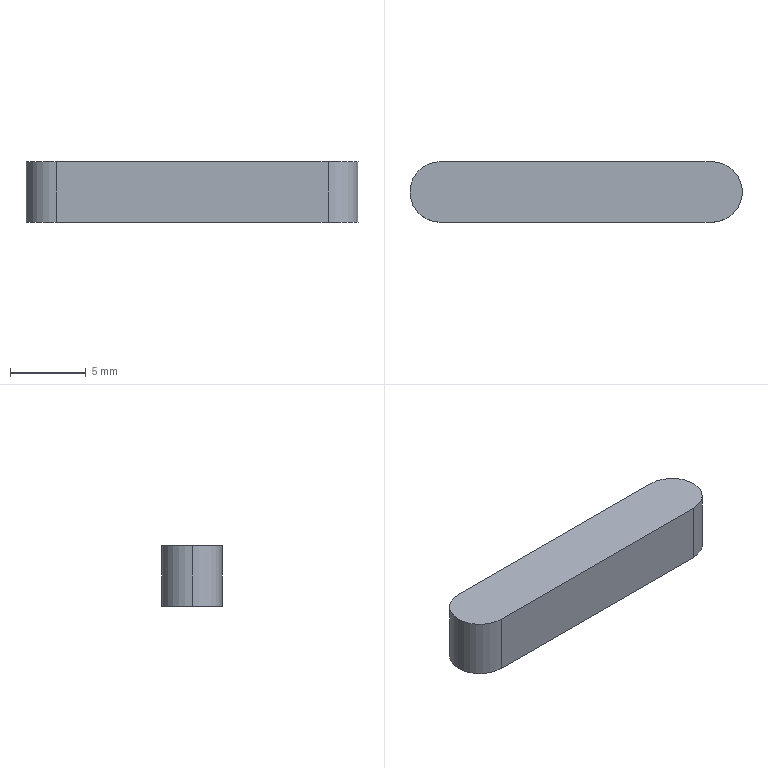Part | SolidWorks | features Extrusion 1 | 1 solid | 7 faces | box 22 x 4 x 4 mm | volume 338.265 mm3 | plane 4 | cylinder 3 | commonest cylinder face diameters 4 x3
STEP:
#1=CARTESIAN_POINT('',(-2.,0.,4.));
#2=VERTEX_POINT('',#1);
#3=CARTESIAN_POINT('',(0.,-2.,4.));
#4=VERTEX_POINT('',#3);
#5=CARTESIAN_POINT('',(0.,0.,4.));
#6=DIRECTION('',(0.,0.,1.));
#7=DIRECTION('',(1.,0.,0.));
#8=AXIS2_PLACEMENT_3D('',#5,#6,#7);
#9=CIRCLE('',#8,2.);
#10=EDGE_CURVE('',#2,#4,#9,.T.);
#11=ORIENTED_EDGE('',*,*,#10,.F.);
#12=CARTESIAN_POINT('',(-2.,0.,0.));
#13=VERTEX_POINT('',#12);
#14=CARTESIAN_POINT('',(-2.,0.,4.));
#15=DIRECTION('',(0.,0.,-1.));
#16=VECTOR('',#15,1000.);
#17=LINE('',#14,#16);
#18=EDGE_CURVE('',#2,#13,#17,.T.);
#19=ORIENTED_EDGE('',*,*,#18,.T.);
#20=CARTESIAN_POINT('',(0.,-2.,0.));
#21=VERTEX_POINT('',#20);
#22=CARTESIAN_POINT('',(0.,0.,0.));
#23=DIRECTION('',(0.,0.,1.));
#24=DIRECTION('',(1.,0.,0.));
#25=AXIS2_PLACEMENT_3D('',#22,#23,#24);
#26=CIRCLE('',#25,2.);
#27=EDGE_CURVE('',#13,#21,#26,.T.);
#28=ORIENTED_EDGE('',*,*,#27,.T.);
#29=CARTESIAN_POINT('',(0.,-2.,4.));
#30=DIRECTION('',(0.,0.,-1.));
#31=VECTOR('',#30,1000.);
#32=LINE('',#29,#31);
#33=EDGE_CURVE('',#4,#21,#32,.T.);
#34=ORIENTED_EDGE('',*,*,#33,.F.);
#35=EDGE_LOOP('',(#11,#19,#28,#34));
#36=FACE_OUTER_BOUND('',#35,.T.);
#37=CARTESIAN_POINT('',(0.,0.,4.));
#38=DIRECTION('',(0.,0.,-1.));
#39=DIRECTION('',(-1.,0.,0.));
#40=AXIS2_PLACEMENT_3D('',#37,#38,#39);
#41=CYLINDRICAL_SURFACE('',#40,2.);
#42=ADVANCED_FACE('',(#36),#41,.T.);
#43=ORIENTED_EDGE('',*,*,#18,.F.);
#44=CARTESIAN_POINT('',(0.,2.,4.));
#45=VERTEX_POINT('',#44);
#46=CARTESIAN_POINT('',(0.,0.,4.));
#47=DIRECTION('',(0.,0.,1.));
#48=DIRECTION('',(1.,0.,0.));
#49=AXIS2_PLACEMENT_3D('',#46,#47,#48);
#50=CIRCLE('',#49,2.);
#51=EDGE_CURVE('',#45,#2,#50,.T.);
#52=ORIENTED_EDGE('',*,*,#51,.F.);
#53=CARTESIAN_POINT('',(0.,2.,0.));
#54=VERTEX_POINT('',#53);
#55=CARTESIAN_POINT('',(0.,2.,4.));
#56=DIRECTION('',(0.,0.,-1.));
#57=VECTOR('',#56,1000.);
#58=LINE('',#55,#57);
#59=EDGE_CURVE('',#45,#54,#58,.T.);
#60=ORIENTED_EDGE('',*,*,#59,.T.);
#61=CARTESIAN_POINT('',(0.,0.,0.));
#62=DIRECTION('',(0.,0.,1.));
#63=DIRECTION('',(1.,0.,0.));
#64=AXIS2_PLACEMENT_3D('',#61,#62,#63);
#65=CIRCLE('',#64,2.);
#66=EDGE_CURVE('',#54,#13,#65,.T.);
#67=ORIENTED_EDGE('',*,*,#66,.T.);
#68=EDGE_LOOP('',(#43,#52,#60,#67));
#69=FACE_OUTER_BOUND('',#68,.T.);
#70=CARTESIAN_POINT('',(0.,0.,4.));
#71=DIRECTION('',(0.,0.,-1.));
#72=DIRECTION('',(-1.,0.,0.));
#73=AXIS2_PLACEMENT_3D('',#70,#71,#72);
#74=CYLINDRICAL_SURFACE('',#73,2.);
#75=ADVANCED_FACE('',(#69),#74,.T.);
#76=CARTESIAN_POINT('',(18.,-2.,0.));
#77=VERTEX_POINT('',#76);
#78=CARTESIAN_POINT('',(0.,-2.,0.));
#79=DIRECTION('',(1.,0.,0.));
#80=VECTOR('',#79,1000.);
#81=LINE('',#78,#80);
#82=EDGE_CURVE('',#21,#77,#81,.T.);
#83=ORIENTED_EDGE('',*,*,#82,.T.);
#84=CARTESIAN_POINT('',(18.,-2.,4.));
#85=VERTEX_POINT('',#84);
#86=CARTESIAN_POINT('',(18.,-2.,4.));
#87=DIRECTION('',(0.,0.,-1.));
#88=VECTOR('',#87,1000.);
#89=LINE('',#86,#88);
#90=EDGE_CURVE('',#85,#77,#89,.T.);
#91=ORIENTED_EDGE('',*,*,#90,.F.);
#92=CARTESIAN_POINT('',(0.,-2.,4.));
#93=DIRECTION('',(1.,0.,0.));
#94=VECTOR('',#93,1000.);
#95=LINE('',#92,#94);
#96=EDGE_CURVE('',#4,#85,#95,.T.);
#97=ORIENTED_EDGE('',*,*,#96,.F.);
#98=ORIENTED_EDGE('',*,*,#33,.T.);
#99=EDGE_LOOP('',(#83,#91,#97,#98));
#100=FACE_OUTER_BOUND('',#99,.T.);
#101=CARTESIAN_POINT('',(0.,-2.,4.));
#102=DIRECTION('',(0.,1.,0.));
#103=DIRECTION('',(0.,0.,1.));
#104=AXIS2_PLACEMENT_3D('',#101,#102,#103);
#105=PLANE('',#104);
#106=ADVANCED_FACE('',(#100),#105,.F.);
#107=CARTESIAN_POINT('',(18.,2.,0.));
#108=VERTEX_POINT('',#107);
#109=CARTESIAN_POINT('',(18.,0.,0.));
#110=DIRECTION('',(0.,0.,1.));
#111=DIRECTION('',(1.,0.,0.));
#112=AXIS2_PLACEMENT_3D('',#109,#110,#111);
#113=CIRCLE('',#112,2.);
#114=EDGE_CURVE('',#77,#108,#113,.T.);
#115=ORIENTED_EDGE('',*,*,#114,.T.);
#116=CARTESIAN_POINT('',(18.,2.,4.));
#117=VERTEX_POINT('',#116);
#118=CARTESIAN_POINT('',(18.,2.,4.));
#119=DIRECTION('',(0.,0.,-1.));
#120=VECTOR('',#119,1000.);
#121=LINE('',#118,#120);
#122=EDGE_CURVE('',#117,#108,#121,.T.);
#123=ORIENTED_EDGE('',*,*,#122,.F.);
#124=CARTESIAN_POINT('',(18.,0.,4.));
#125=DIRECTION('',(0.,0.,1.));
#126=DIRECTION('',(1.,0.,0.));
#127=AXIS2_PLACEMENT_3D('',#124,#125,#126);
#128=CIRCLE('',#127,2.);
#129=EDGE_CURVE('',#85,#117,#128,.T.);
#130=ORIENTED_EDGE('',*,*,#129,.F.);
#131=ORIENTED_EDGE('',*,*,#90,.T.);
#132=EDGE_LOOP('',(#115,#123,#130,#131));
#133=FACE_OUTER_BOUND('',#132,.T.);
#134=CARTESIAN_POINT('',(18.,0.,4.));
#135=DIRECTION('',(0.,0.,-1.));
#136=DIRECTION('',(-1.,0.,0.));
#137=AXIS2_PLACEMENT_3D('',#134,#135,#136);
#138=CYLINDRICAL_SURFACE('',#137,2.);
#139=ADVANCED_FACE('',(#133),#138,.T.);
#140=CARTESIAN_POINT('',(0.,2.,0.));
#141=DIRECTION('',(-1.,0.,0.));
#142=VECTOR('',#141,1000.);
#143=LINE('',#140,#142);
#144=EDGE_CURVE('',#108,#54,#143,.T.);
#145=ORIENTED_EDGE('',*,*,#144,.T.);
#146=ORIENTED_EDGE('',*,*,#59,.F.);
#147=CARTESIAN_POINT('',(0.,2.,4.));
#148=DIRECTION('',(-1.,0.,0.));
#149=VECTOR('',#148,1000.);
#150=LINE('',#147,#149);
#151=EDGE_CURVE('',#117,#45,#150,.T.);
#152=ORIENTED_EDGE('',*,*,#151,.F.);
#153=ORIENTED_EDGE('',*,*,#122,.T.);
#154=EDGE_LOOP('',(#145,#146,#152,#153));
#155=FACE_OUTER_BOUND('',#154,.T.);
#156=CARTESIAN_POINT('',(0.,2.,4.));
#157=DIRECTION('',(0.,-1.,0.));
#158=DIRECTION('',(0.,0.,-1.));
#159=AXIS2_PLACEMENT_3D('',#156,#157,#158);
#160=PLANE('',#159);
#161=ADVANCED_FACE('',(#155),#160,.F.);
#162=ORIENTED_EDGE('',*,*,#51,.T.);
#163=ORIENTED_EDGE('',*,*,#10,.T.);
#164=ORIENTED_EDGE('',*,*,#96,.T.);
#165=ORIENTED_EDGE('',*,*,#129,.T.);
#166=ORIENTED_EDGE('',*,*,#151,.T.);
#167=EDGE_LOOP('',(#162,#163,#164,#165,#166));
#168=FACE_OUTER_BOUND('',#167,.T.);
#169=CARTESIAN_POINT('',(0.,0.,4.));
#170=DIRECTION('',(0.,0.,1.));
#171=DIRECTION('',(1.,0.,0.));
#172=AXIS2_PLACEMENT_3D('',#169,#170,#171);
#173=PLANE('',#172);
#174=ADVANCED_FACE('',(#168),#173,.T.);
#175=ORIENTED_EDGE('',*,*,#66,.F.);
#176=ORIENTED_EDGE('',*,*,#144,.F.);
#177=ORIENTED_EDGE('',*,*,#114,.F.);
#178=ORIENTED_EDGE('',*,*,#82,.F.);
#179=ORIENTED_EDGE('',*,*,#27,.F.);
#180=EDGE_LOOP('',(#175,#176,#177,#178,#179));
#181=FACE_OUTER_BOUND('',#180,.T.);
#182=CARTESIAN_POINT('',(0.,0.,0.));
#183=DIRECTION('',(0.,0.,1.));
#184=DIRECTION('',(1.,0.,0.));
#185=AXIS2_PLACEMENT_3D('',#182,#183,#184);
#186=PLANE('',#185);
#187=ADVANCED_FACE('',(#181),#186,.F.);
#188=CLOSED_SHELL('',(#42,#75,#106,#139,#161,#174,#187));
#189=MANIFOLD_SOLID_BREP('',#188);
#190=CARTESIAN_POINT('',(0.,0.,0.));
#191=DIRECTION('',(0.,0.,1.));
#192=DIRECTION('',(1.,0.,0.));
#193=AXIS2_PLACEMENT_3D('',#190,#191,#192);
#194=(LENGTH_UNIT()NAMED_UNIT(*)SI_UNIT(.MILLI.,.METRE.));
#195=UNCERTAINTY_MEASURE_WITH_UNIT(LENGTH_MEASURE(0.00001),#194,'','');
#196=(NAMED_UNIT(*)PLANE_ANGLE_UNIT()SI_UNIT($,.RADIAN.));
#197=(NAMED_UNIT(*)SI_UNIT($,.STERADIAN.)SOLID_ANGLE_UNIT());
#198=(GEOMETRIC_REPRESENTATION_CONTEXT(3)GLOBAL_UNCERTAINTY_ASSIGNED_CONTEXT((#195))GLOBAL_UNIT_ASSIGNED_CONTEXT((#194,#196,#197))REPRESENTATION_CONTEXT('',''));
#199=ADVANCED_BREP_SHAPE_REPRESENTATION('',(#189,#193),#198);